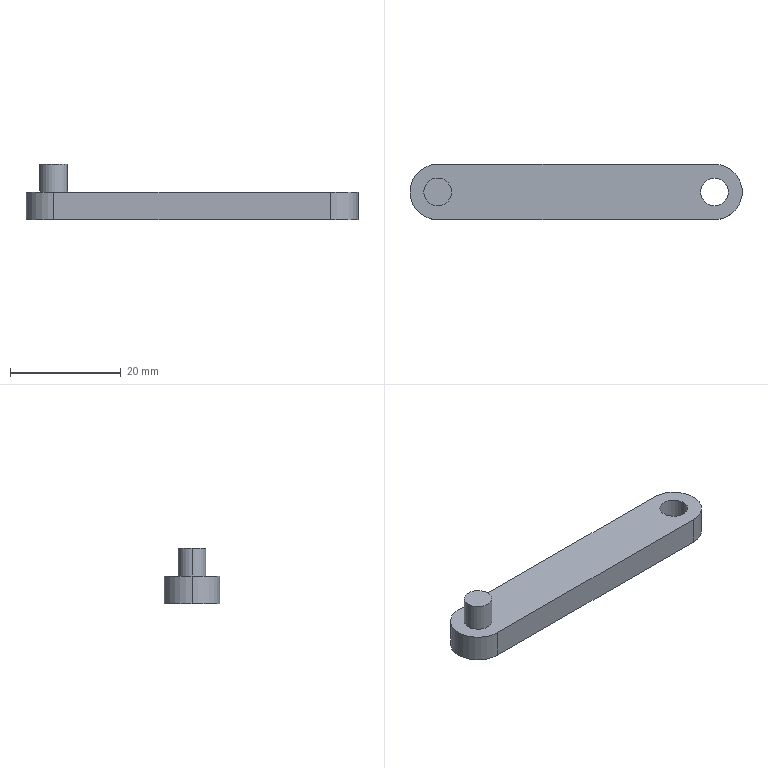Part | SolidWorks | 1 solid | 12 faces | box 60 x 10 x 10 mm | volume 2893 mm3 | cylinder 7 | plane 5 | commonest cylinder face diameters 5 x4 10 x3
STEP:
#1=CARTESIAN_POINT('',(-22.5,0.,10.));
#2=VERTEX_POINT('',#1);
#3=CARTESIAN_POINT('',(-27.5,0.,10.));
#4=VERTEX_POINT('',#3);
#5=CARTESIAN_POINT('',(-25.,0.,10.));
#6=DIRECTION('',(0.,0.,1.));
#7=DIRECTION('',(1.,0.,0.));
#8=AXIS2_PLACEMENT_3D('',#5,#6,#7);
#9=CIRCLE('',#8,2.5);
#10=EDGE_CURVE('',#2,#4,#9,.T.);
#11=ORIENTED_EDGE('',*,*,#10,.F.);
#12=CARTESIAN_POINT('',(-22.5,0.,5.));
#13=VERTEX_POINT('',#12);
#14=CARTESIAN_POINT('',(-22.5,0.,10.));
#15=DIRECTION('',(0.,0.,-1.));
#16=VECTOR('',#15,1000.);
#17=LINE('',#14,#16);
#18=EDGE_CURVE('',#2,#13,#17,.T.);
#19=ORIENTED_EDGE('',*,*,#18,.T.);
#20=CARTESIAN_POINT('',(-27.5,0.,5.));
#21=VERTEX_POINT('',#20);
#22=CARTESIAN_POINT('',(-25.,0.,5.));
#23=DIRECTION('',(0.,0.,1.));
#24=DIRECTION('',(1.,0.,0.));
#25=AXIS2_PLACEMENT_3D('',#22,#23,#24);
#26=CIRCLE('',#25,2.5);
#27=EDGE_CURVE('',#13,#21,#26,.T.);
#28=ORIENTED_EDGE('',*,*,#27,.T.);
#29=CARTESIAN_POINT('',(-27.5,0.,10.));
#30=DIRECTION('',(0.,0.,-1.));
#31=VECTOR('',#30,1000.);
#32=LINE('',#29,#31);
#33=EDGE_CURVE('',#4,#21,#32,.T.);
#34=ORIENTED_EDGE('',*,*,#33,.F.);
#35=EDGE_LOOP('',(#11,#19,#28,#34));
#36=FACE_OUTER_BOUND('',#35,.T.);
#37=CARTESIAN_POINT('',(-25.,0.,10.));
#38=DIRECTION('',(0.,0.,-1.));
#39=DIRECTION('',(-1.,0.,0.));
#40=AXIS2_PLACEMENT_3D('',#37,#38,#39);
#41=CYLINDRICAL_SURFACE('',#40,2.5);
#42=ADVANCED_FACE('',(#36),#41,.T.);
#43=CARTESIAN_POINT('',(22.5,0.,0.));
#44=VERTEX_POINT('',#43);
#45=CARTESIAN_POINT('',(27.5,0.,0.));
#46=VERTEX_POINT('',#45);
#47=CARTESIAN_POINT('',(25.,0.,0.));
#48=DIRECTION('',(0.,0.,1.));
#49=DIRECTION('',(1.,0.,0.));
#50=AXIS2_PLACEMENT_3D('',#47,#48,#49);
#51=CIRCLE('',#50,2.5);
#52=EDGE_CURVE('',#44,#46,#51,.T.);
#53=ORIENTED_EDGE('',*,*,#52,.F.);
#54=CARTESIAN_POINT('',(22.5,0.,5.));
#55=VERTEX_POINT('',#54);
#56=CARTESIAN_POINT('',(22.5,0.,0.));
#57=DIRECTION('',(0.,0.,1.));
#58=VECTOR('',#57,1000.);
#59=LINE('',#56,#58);
#60=EDGE_CURVE('',#44,#55,#59,.T.);
#61=ORIENTED_EDGE('',*,*,#60,.T.);
#62=CARTESIAN_POINT('',(27.5,0.,5.));
#63=VERTEX_POINT('',#62);
#64=CARTESIAN_POINT('',(25.,0.,5.));
#65=DIRECTION('',(0.,0.,1.));
#66=DIRECTION('',(1.,0.,0.));
#67=AXIS2_PLACEMENT_3D('',#64,#65,#66);
#68=CIRCLE('',#67,2.5);
#69=EDGE_CURVE('',#55,#63,#68,.T.);
#70=ORIENTED_EDGE('',*,*,#69,.T.);
#71=CARTESIAN_POINT('',(27.5,0.,0.));
#72=DIRECTION('',(0.,0.,1.));
#73=VECTOR('',#72,1000.);
#74=LINE('',#71,#73);
#75=EDGE_CURVE('',#46,#63,#74,.T.);
#76=ORIENTED_EDGE('',*,*,#75,.F.);
#77=EDGE_LOOP('',(#53,#61,#70,#76));
#78=FACE_OUTER_BOUND('',#77,.T.);
#79=CARTESIAN_POINT('',(25.,0.,0.));
#80=DIRECTION('',(0.,0.,1.));
#81=DIRECTION('',(1.,0.,0.));
#82=AXIS2_PLACEMENT_3D('',#79,#80,#81);
#83=CYLINDRICAL_SURFACE('',#82,2.5);
#84=ADVANCED_FACE('',(#78),#83,.F.);
#85=CARTESIAN_POINT('',(-30.,0.,5.));
#86=VERTEX_POINT('',#85);
#87=CARTESIAN_POINT('',(-25.,-5.,5.));
#88=VERTEX_POINT('',#87);
#89=CARTESIAN_POINT('',(-25.,0.,5.));
#90=DIRECTION('',(0.,0.,1.));
#91=DIRECTION('',(1.,0.,0.));
#92=AXIS2_PLACEMENT_3D('',#89,#90,#91);
#93=CIRCLE('',#92,5.);
#94=EDGE_CURVE('',#86,#88,#93,.T.);
#95=ORIENTED_EDGE('',*,*,#94,.F.);
#96=CARTESIAN_POINT('',(-30.,0.,0.));
#97=VERTEX_POINT('',#96);
#98=CARTESIAN_POINT('',(-30.,0.,5.));
#99=DIRECTION('',(0.,0.,-1.));
#100=VECTOR('',#99,1000.);
#101=LINE('',#98,#100);
#102=EDGE_CURVE('',#86,#97,#101,.T.);
#103=ORIENTED_EDGE('',*,*,#102,.T.);
#104=CARTESIAN_POINT('',(-25.,-5.,0.));
#105=VERTEX_POINT('',#104);
#106=CARTESIAN_POINT('',(-25.,0.,0.));
#107=DIRECTION('',(0.,0.,1.));
#108=DIRECTION('',(1.,0.,0.));
#109=AXIS2_PLACEMENT_3D('',#106,#107,#108);
#110=CIRCLE('',#109,5.);
#111=EDGE_CURVE('',#97,#105,#110,.T.);
#112=ORIENTED_EDGE('',*,*,#111,.T.);
#113=CARTESIAN_POINT('',(-25.,-5.,5.));
#114=DIRECTION('',(0.,0.,-1.));
#115=VECTOR('',#114,1000.);
#116=LINE('',#113,#115);
#117=EDGE_CURVE('',#88,#105,#116,.T.);
#118=ORIENTED_EDGE('',*,*,#117,.F.);
#119=EDGE_LOOP('',(#95,#103,#112,#118));
#120=FACE_OUTER_BOUND('',#119,.T.);
#121=CARTESIAN_POINT('',(-25.,0.,5.));
#122=DIRECTION('',(0.,0.,-1.));
#123=DIRECTION('',(-1.,0.,0.));
#124=AXIS2_PLACEMENT_3D('',#121,#122,#123);
#125=CYLINDRICAL_SURFACE('',#124,5.);
#126=ADVANCED_FACE('',(#120),#125,.T.);
#127=ORIENTED_EDGE('',*,*,#102,.F.);
#128=CARTESIAN_POINT('',(-25.,5.,5.));
#129=VERTEX_POINT('',#128);
#130=CARTESIAN_POINT('',(-25.,0.,5.));
#131=DIRECTION('',(0.,0.,1.));
#132=DIRECTION('',(1.,0.,0.));
#133=AXIS2_PLACEMENT_3D('',#130,#131,#132);
#134=CIRCLE('',#133,5.);
#135=EDGE_CURVE('',#129,#86,#134,.T.);
#136=ORIENTED_EDGE('',*,*,#135,.F.);
#137=CARTESIAN_POINT('',(-25.,5.,0.));
#138=VERTEX_POINT('',#137);
#139=CARTESIAN_POINT('',(-25.,5.,5.));
#140=DIRECTION('',(0.,0.,-1.));
#141=VECTOR('',#140,1000.);
#142=LINE('',#139,#141);
#143=EDGE_CURVE('',#129,#138,#142,.T.);
#144=ORIENTED_EDGE('',*,*,#143,.T.);
#145=CARTESIAN_POINT('',(-25.,0.,0.));
#146=DIRECTION('',(0.,0.,1.));
#147=DIRECTION('',(1.,0.,0.));
#148=AXIS2_PLACEMENT_3D('',#145,#146,#147);
#149=CIRCLE('',#148,5.);
#150=EDGE_CURVE('',#138,#97,#149,.T.);
#151=ORIENTED_EDGE('',*,*,#150,.T.);
#152=EDGE_LOOP('',(#127,#136,#144,#151));
#153=FACE_OUTER_BOUND('',#152,.T.);
#154=CARTESIAN_POINT('',(-25.,0.,5.));
#155=DIRECTION('',(0.,0.,-1.));
#156=DIRECTION('',(-1.,0.,0.));
#157=AXIS2_PLACEMENT_3D('',#154,#155,#156);
#158=CYLINDRICAL_SURFACE('',#157,5.);
#159=ADVANCED_FACE('',(#153),#158,.T.);
#160=CARTESIAN_POINT('',(25.,-5.,0.));
#161=VERTEX_POINT('',#160);
#162=CARTESIAN_POINT('',(-25.,-5.,0.));
#163=DIRECTION('',(1.,0.,0.));
#164=VECTOR('',#163,1000.);
#165=LINE('',#162,#164);
#166=EDGE_CURVE('',#105,#161,#165,.T.);
#167=ORIENTED_EDGE('',*,*,#166,.T.);
#168=CARTESIAN_POINT('',(25.,-5.,5.));
#169=VERTEX_POINT('',#168);
#170=CARTESIAN_POINT('',(25.,-5.,5.));
#171=DIRECTION('',(0.,0.,-1.));
#172=VECTOR('',#171,1000.);
#173=LINE('',#170,#172);
#174=EDGE_CURVE('',#169,#161,#173,.T.);
#175=ORIENTED_EDGE('',*,*,#174,.F.);
#176=CARTESIAN_POINT('',(-25.,-5.,5.));
#177=DIRECTION('',(1.,0.,0.));
#178=VECTOR('',#177,1000.);
#179=LINE('',#176,#178);
#180=EDGE_CURVE('',#88,#169,#179,.T.);
#181=ORIENTED_EDGE('',*,*,#180,.F.);
#182=ORIENTED_EDGE('',*,*,#117,.T.);
#183=EDGE_LOOP('',(#167,#175,#181,#182));
#184=FACE_OUTER_BOUND('',#183,.T.);
#185=CARTESIAN_POINT('',(-25.,-5.,5.));
#186=DIRECTION('',(0.,1.,0.));
#187=DIRECTION('',(-1.,0.,0.));
#188=AXIS2_PLACEMENT_3D('',#185,#186,#187);
#189=PLANE('',#188);
#190=ADVANCED_FACE('',(#184),#189,.F.);
#191=CARTESIAN_POINT('',(25.,5.,0.));
#192=VERTEX_POINT('',#191);
#193=CARTESIAN_POINT('',(25.,0.,0.));
#194=DIRECTION('',(0.,0.,1.));
#195=DIRECTION('',(1.,0.,0.));
#196=AXIS2_PLACEMENT_3D('',#193,#194,#195);
#197=CIRCLE('',#196,5.);
#198=EDGE_CURVE('',#161,#192,#197,.T.);
#199=ORIENTED_EDGE('',*,*,#198,.T.);
#200=CARTESIAN_POINT('',(25.,5.,5.));
#201=VERTEX_POINT('',#200);
#202=CARTESIAN_POINT('',(25.,5.,5.));
#203=DIRECTION('',(0.,0.,-1.));
#204=VECTOR('',#203,1000.);
#205=LINE('',#202,#204);
#206=EDGE_CURVE('',#201,#192,#205,.T.);
#207=ORIENTED_EDGE('',*,*,#206,.F.);
#208=CARTESIAN_POINT('',(25.,0.,5.));
#209=DIRECTION('',(0.,0.,1.));
#210=DIRECTION('',(1.,0.,0.));
#211=AXIS2_PLACEMENT_3D('',#208,#209,#210);
#212=CIRCLE('',#211,5.);
#213=EDGE_CURVE('',#169,#201,#212,.T.);
#214=ORIENTED_EDGE('',*,*,#213,.F.);
#215=ORIENTED_EDGE('',*,*,#174,.T.);
#216=EDGE_LOOP('',(#199,#207,#214,#215));
#217=FACE_OUTER_BOUND('',#216,.T.);
#218=CARTESIAN_POINT('',(25.,0.,5.));
#219=DIRECTION('',(0.,0.,-1.));
#220=DIRECTION('',(-1.,0.,0.));
#221=AXIS2_PLACEMENT_3D('',#218,#219,#220);
#222=CYLINDRICAL_SURFACE('',#221,5.);
#223=ADVANCED_FACE('',(#217),#222,.T.);
#224=CARTESIAN_POINT('',(-25.,5.,0.));
#225=DIRECTION('',(-1.,0.,0.));
#226=VECTOR('',#225,1000.);
#227=LINE('',#224,#226);
#228=EDGE_CURVE('',#192,#138,#227,.T.);
#229=ORIENTED_EDGE('',*,*,#228,.T.);
#230=ORIENTED_EDGE('',*,*,#143,.F.);
#231=CARTESIAN_POINT('',(-25.,5.,5.));
#232=DIRECTION('',(-1.,0.,0.));
#233=VECTOR('',#232,1000.);
#234=LINE('',#231,#233);
#235=EDGE_CURVE('',#201,#129,#234,.T.);
#236=ORIENTED_EDGE('',*,*,#235,.F.);
#237=ORIENTED_EDGE('',*,*,#206,.T.);
#238=EDGE_LOOP('',(#229,#230,#236,#237));
#239=FACE_OUTER_BOUND('',#238,.T.);
#240=CARTESIAN_POINT('',(-25.,5.,5.));
#241=DIRECTION('',(0.,-1.,0.));
#242=DIRECTION('',(1.,0.,0.));
#243=AXIS2_PLACEMENT_3D('',#240,#241,#242);
#244=PLANE('',#243);
#245=ADVANCED_FACE('',(#239),#244,.F.);
#246=CARTESIAN_POINT('',(-25.,0.,5.));
#247=DIRECTION('',(0.,0.,1.));
#248=DIRECTION('',(1.,0.,0.));
#249=AXIS2_PLACEMENT_3D('',#246,#247,#248);
#250=CIRCLE('',#249,2.5);
#251=EDGE_CURVE('',#21,#13,#250,.T.);
#252=ORIENTED_EDGE('',*,*,#251,.F.);
#253=ORIENTED_EDGE('',*,*,#27,.F.);
#254=EDGE_LOOP('',(#252,#253));
#255=FACE_BOUND('',#254,.T.);
#256=CARTESIAN_POINT('',(25.,0.,5.));
#257=DIRECTION('',(0.,0.,1.));
#258=DIRECTION('',(1.,0.,0.));
#259=AXIS2_PLACEMENT_3D('',#256,#257,#258);
#260=CIRCLE('',#259,2.5);
#261=EDGE_CURVE('',#63,#55,#260,.T.);
#262=ORIENTED_EDGE('',*,*,#261,.F.);
#263=ORIENTED_EDGE('',*,*,#69,.F.);
#264=EDGE_LOOP('',(#262,#263));
#265=FACE_BOUND('',#264,.T.);
#266=ORIENTED_EDGE('',*,*,#135,.T.);
#267=ORIENTED_EDGE('',*,*,#94,.T.);
#268=ORIENTED_EDGE('',*,*,#180,.T.);
#269=ORIENTED_EDGE('',*,*,#213,.T.);
#270=ORIENTED_EDGE('',*,*,#235,.T.);
#271=EDGE_LOOP('',(#266,#267,#268,#269,#270));
#272=FACE_OUTER_BOUND('',#271,.T.);
#273=CARTESIAN_POINT('',(-25.,0.,5.));
#274=DIRECTION('',(0.,0.,1.));
#275=DIRECTION('',(1.,0.,0.));
#276=AXIS2_PLACEMENT_3D('',#273,#274,#275);
#277=PLANE('',#276);
#278=ADVANCED_FACE('',(#255,#265,#272),#277,.T.);
#279=CARTESIAN_POINT('',(25.,0.,0.));
#280=DIRECTION('',(0.,0.,1.));
#281=DIRECTION('',(1.,0.,0.));
#282=AXIS2_PLACEMENT_3D('',#279,#280,#281);
#283=CIRCLE('',#282,2.5);
#284=EDGE_CURVE('',#46,#44,#283,.T.);
#285=ORIENTED_EDGE('',*,*,#284,.T.);
#286=ORIENTED_EDGE('',*,*,#52,.T.);
#287=EDGE_LOOP('',(#285,#286));
#288=FACE_BOUND('',#287,.T.);
#289=ORIENTED_EDGE('',*,*,#150,.F.);
#290=ORIENTED_EDGE('',*,*,#228,.F.);
#291=ORIENTED_EDGE('',*,*,#198,.F.);
#292=ORIENTED_EDGE('',*,*,#166,.F.);
#293=ORIENTED_EDGE('',*,*,#111,.F.);
#294=EDGE_LOOP('',(#289,#290,#291,#292,#293));
#295=FACE_OUTER_BOUND('',#294,.T.);
#296=CARTESIAN_POINT('',(-25.,0.,0.));
#297=DIRECTION('',(0.,0.,1.));
#298=DIRECTION('',(1.,0.,0.));
#299=AXIS2_PLACEMENT_3D('',#296,#297,#298);
#300=PLANE('',#299);
#301=ADVANCED_FACE('',(#288,#295),#300,.F.);
#302=ORIENTED_EDGE('',*,*,#60,.F.);
#303=ORIENTED_EDGE('',*,*,#284,.F.);
#304=ORIENTED_EDGE('',*,*,#75,.T.);
#305=ORIENTED_EDGE('',*,*,#261,.T.);
#306=EDGE_LOOP('',(#302,#303,#304,#305));
#307=FACE_OUTER_BOUND('',#306,.T.);
#308=CARTESIAN_POINT('',(25.,0.,0.));
#309=DIRECTION('',(0.,0.,1.));
#310=DIRECTION('',(1.,0.,0.));
#311=AXIS2_PLACEMENT_3D('',#308,#309,#310);
#312=CYLINDRICAL_SURFACE('',#311,2.5);
#313=ADVANCED_FACE('',(#307),#312,.F.);
#314=ORIENTED_EDGE('',*,*,#18,.F.);
#315=CARTESIAN_POINT('',(-25.,0.,10.));
#316=DIRECTION('',(0.,0.,1.));
#317=DIRECTION('',(1.,0.,0.));
#318=AXIS2_PLACEMENT_3D('',#315,#316,#317);
#319=CIRCLE('',#318,2.5);
#320=EDGE_CURVE('',#4,#2,#319,.T.);
#321=ORIENTED_EDGE('',*,*,#320,.F.);
#322=ORIENTED_EDGE('',*,*,#33,.T.);
#323=ORIENTED_EDGE('',*,*,#251,.T.);
#324=EDGE_LOOP('',(#314,#321,#322,#323));
#325=FACE_OUTER_BOUND('',#324,.T.);
#326=CARTESIAN_POINT('',(-25.,0.,10.));
#327=DIRECTION('',(0.,0.,-1.));
#328=DIRECTION('',(-1.,0.,0.));
#329=AXIS2_PLACEMENT_3D('',#326,#327,#328);
#330=CYLINDRICAL_SURFACE('',#329,2.5);
#331=ADVANCED_FACE('',(#325),#330,.T.);
#332=ORIENTED_EDGE('',*,*,#320,.T.);
#333=ORIENTED_EDGE('',*,*,#10,.T.);
#334=EDGE_LOOP('',(#332,#333));
#335=FACE_OUTER_BOUND('',#334,.T.);
#336=CARTESIAN_POINT('',(-25.,0.,10.));
#337=DIRECTION('',(0.,0.,1.));
#338=DIRECTION('',(1.,0.,0.));
#339=AXIS2_PLACEMENT_3D('',#336,#337,#338);
#340=PLANE('',#339);
#341=ADVANCED_FACE('',(#335),#340,.T.);
#342=CLOSED_SHELL('',(#42,#84,#126,#159,#190,#223,#245,#278,#301,#313,#331,#341));
#343=MANIFOLD_SOLID_BREP('',#342);
#344=CARTESIAN_POINT('',(0.,0.,0.));
#345=DIRECTION('',(0.,0.,1.));
#346=DIRECTION('',(1.,0.,0.));
#347=AXIS2_PLACEMENT_3D('',#344,#345,#346);
#348=(LENGTH_UNIT()NAMED_UNIT(*)SI_UNIT(.MILLI.,.METRE.));
#349=UNCERTAINTY_MEASURE_WITH_UNIT(LENGTH_MEASURE(0.00001),#348,'','');
#350=(NAMED_UNIT(*)PLANE_ANGLE_UNIT()SI_UNIT($,.RADIAN.));
#351=(NAMED_UNIT(*)SI_UNIT($,.STERADIAN.)SOLID_ANGLE_UNIT());
#352=(GEOMETRIC_REPRESENTATION_CONTEXT(3)GLOBAL_UNCERTAINTY_ASSIGNED_CONTEXT((#349))GLOBAL_UNIT_ASSIGNED_CONTEXT((#348,#350,#351))REPRESENTATION_CONTEXT('',''));
#353=ADVANCED_BREP_SHAPE_REPRESENTATION('',(#343,#347),#352);